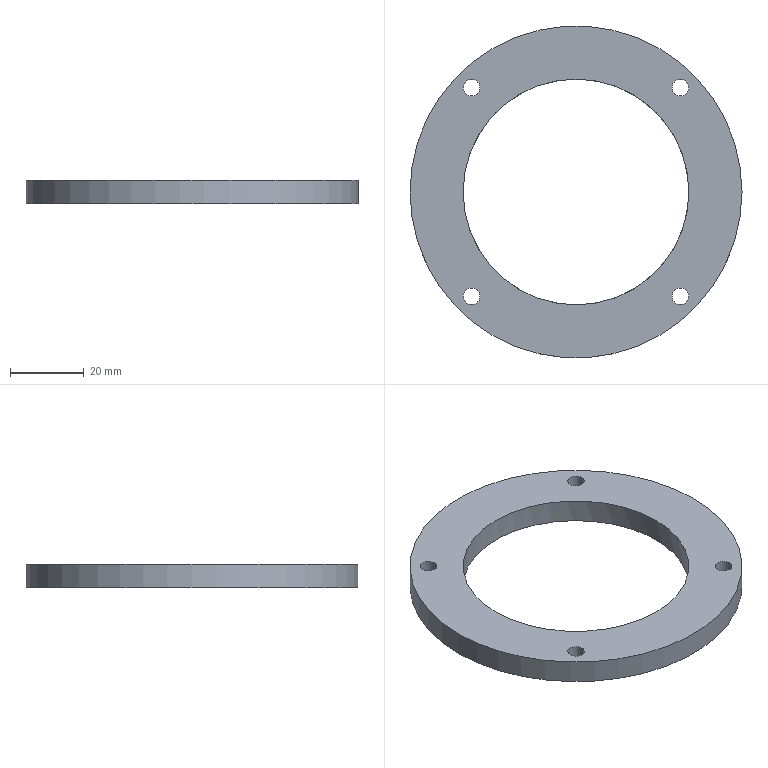Part | NX | features DATUM_CSYS 1, EXTRUDE 1, LINKED_FACE 1, SKETCH 1 | 1 solid | 8 faces | box 90 x 90 x 6.5 mm | volume 21817 mm3 | cylinder 6 | plane 2 | commonest cylinder face diameters 4.5 x4 61.2 x1 90 x1
STEP:
#1=CARTESIAN_POINT('',(-26.034,-28.284,0.));
#2=VERTEX_POINT('',#1);
#3=CARTESIAN_POINT('',(-28.284,-28.284,0.));
#4=DIRECTION('',(0.,0.,1.));
#5=DIRECTION('',(1.,0.,0.));
#6=AXIS2_PLACEMENT_3D('',#3,#4,#5);
#7=CIRCLE('',#6,2.25);
#8=EDGE_CURVE('',#2,#2,#7,.T.);
#9=ORIENTED_EDGE('',*,*,#8,.F.);
#10=EDGE_LOOP('',(#9));
#11=FACE_BOUND('',#10,.T.);
#12=CARTESIAN_POINT('',(-30.534,-28.284,6.5));
#13=VERTEX_POINT('',#12);
#14=CARTESIAN_POINT('',(-28.284,-28.284,6.5));
#15=DIRECTION('',(0.,0.,1.));
#16=DIRECTION('',(-1.,0.,0.));
#17=AXIS2_PLACEMENT_3D('',#14,#15,#16);
#18=CIRCLE('',#17,2.25);
#19=EDGE_CURVE('',#13,#13,#18,.T.);
#20=ORIENTED_EDGE('',*,*,#19,.T.);
#21=EDGE_LOOP('',(#20));
#22=FACE_BOUND('',#21,.T.);
#23=CARTESIAN_POINT('',(-28.284,-28.284,6.5));
#24=DIRECTION('',(0.,0.,-1.));
#25=DIRECTION('',(-1.,0.,0.));
#26=AXIS2_PLACEMENT_3D('',#23,#24,#25);
#27=CYLINDRICAL_SURFACE('',#26,2.25);
#28=ADVANCED_FACE('',(#11,#22),#27,.F.);
#29=CARTESIAN_POINT('',(-26.034,28.284,0.));
#30=VERTEX_POINT('',#29);
#31=CARTESIAN_POINT('',(-28.284,28.284,0.));
#32=DIRECTION('',(0.,0.,1.));
#33=DIRECTION('',(1.,0.,0.));
#34=AXIS2_PLACEMENT_3D('',#31,#32,#33);
#35=CIRCLE('',#34,2.25);
#36=EDGE_CURVE('',#30,#30,#35,.T.);
#37=ORIENTED_EDGE('',*,*,#36,.F.);
#38=EDGE_LOOP('',(#37));
#39=FACE_BOUND('',#38,.T.);
#40=CARTESIAN_POINT('',(-30.534,28.284,6.5));
#41=VERTEX_POINT('',#40);
#42=CARTESIAN_POINT('',(-28.284,28.284,6.5));
#43=DIRECTION('',(0.,0.,1.));
#44=DIRECTION('',(-1.,0.,0.));
#45=AXIS2_PLACEMENT_3D('',#42,#43,#44);
#46=CIRCLE('',#45,2.25);
#47=EDGE_CURVE('',#41,#41,#46,.T.);
#48=ORIENTED_EDGE('',*,*,#47,.T.);
#49=EDGE_LOOP('',(#48));
#50=FACE_BOUND('',#49,.T.);
#51=CARTESIAN_POINT('',(-28.284,28.284,6.5));
#52=DIRECTION('',(0.,0.,-1.));
#53=DIRECTION('',(-1.,0.,0.));
#54=AXIS2_PLACEMENT_3D('',#51,#52,#53);
#55=CYLINDRICAL_SURFACE('',#54,2.25);
#56=ADVANCED_FACE('',(#39,#50),#55,.F.);
#57=CARTESIAN_POINT('',(30.534,-28.284,0.));
#58=VERTEX_POINT('',#57);
#59=CARTESIAN_POINT('',(28.284,-28.284,0.));
#60=DIRECTION('',(0.,0.,1.));
#61=DIRECTION('',(1.,0.,0.));
#62=AXIS2_PLACEMENT_3D('',#59,#60,#61);
#63=CIRCLE('',#62,2.25);
#64=EDGE_CURVE('',#58,#58,#63,.T.);
#65=ORIENTED_EDGE('',*,*,#64,.F.);
#66=EDGE_LOOP('',(#65));
#67=FACE_BOUND('',#66,.T.);
#68=CARTESIAN_POINT('',(26.034,-28.284,6.5));
#69=VERTEX_POINT('',#68);
#70=CARTESIAN_POINT('',(28.284,-28.284,6.5));
#71=DIRECTION('',(0.,0.,1.));
#72=DIRECTION('',(-1.,0.,0.));
#73=AXIS2_PLACEMENT_3D('',#70,#71,#72);
#74=CIRCLE('',#73,2.25);
#75=EDGE_CURVE('',#69,#69,#74,.T.);
#76=ORIENTED_EDGE('',*,*,#75,.T.);
#77=EDGE_LOOP('',(#76));
#78=FACE_BOUND('',#77,.T.);
#79=CARTESIAN_POINT('',(28.284,-28.284,6.5));
#80=DIRECTION('',(0.,0.,-1.));
#81=DIRECTION('',(-1.,0.,0.));
#82=AXIS2_PLACEMENT_3D('',#79,#80,#81);
#83=CYLINDRICAL_SURFACE('',#82,2.25);
#84=ADVANCED_FACE('',(#67,#78),#83,.F.);
#85=CARTESIAN_POINT('',(30.534,28.284,0.));
#86=VERTEX_POINT('',#85);
#87=CARTESIAN_POINT('',(28.284,28.284,0.));
#88=DIRECTION('',(0.,0.,1.));
#89=DIRECTION('',(1.,0.,0.));
#90=AXIS2_PLACEMENT_3D('',#87,#88,#89);
#91=CIRCLE('',#90,2.25);
#92=EDGE_CURVE('',#86,#86,#91,.T.);
#93=ORIENTED_EDGE('',*,*,#92,.F.);
#94=EDGE_LOOP('',(#93));
#95=FACE_BOUND('',#94,.T.);
#96=CARTESIAN_POINT('',(26.034,28.284,6.5));
#97=VERTEX_POINT('',#96);
#98=CARTESIAN_POINT('',(28.284,28.284,6.5));
#99=DIRECTION('',(0.,0.,1.));
#100=DIRECTION('',(-1.,0.,0.));
#101=AXIS2_PLACEMENT_3D('',#98,#99,#100);
#102=CIRCLE('',#101,2.25);
#103=EDGE_CURVE('',#97,#97,#102,.T.);
#104=ORIENTED_EDGE('',*,*,#103,.T.);
#105=EDGE_LOOP('',(#104));
#106=FACE_BOUND('',#105,.T.);
#107=CARTESIAN_POINT('',(28.284,28.284,6.5));
#108=DIRECTION('',(0.,0.,-1.));
#109=DIRECTION('',(-1.,0.,0.));
#110=AXIS2_PLACEMENT_3D('',#107,#108,#109);
#111=CYLINDRICAL_SURFACE('',#110,2.25);
#112=ADVANCED_FACE('',(#95,#106),#111,.F.);
#113=CARTESIAN_POINT('',(-45.,0.,0.));
#114=VERTEX_POINT('',#113);
#115=CARTESIAN_POINT('',(0.,0.,0.));
#116=DIRECTION('',(0.,0.,-1.));
#117=DIRECTION('',(-1.,0.,0.));
#118=AXIS2_PLACEMENT_3D('',#115,#116,#117);
#119=CIRCLE('',#118,45.);
#120=EDGE_CURVE('',#114,#114,#119,.T.);
#121=ORIENTED_EDGE('',*,*,#120,.F.);
#122=EDGE_LOOP('',(#121));
#123=FACE_BOUND('',#122,.T.);
#124=CARTESIAN_POINT('',(45.,0.,6.5));
#125=VERTEX_POINT('',#124);
#126=CARTESIAN_POINT('',(0.,0.,6.5));
#127=DIRECTION('',(0.,0.,-1.));
#128=DIRECTION('',(1.,0.,0.));
#129=AXIS2_PLACEMENT_3D('',#126,#127,#128);
#130=CIRCLE('',#129,45.);
#131=EDGE_CURVE('',#125,#125,#130,.T.);
#132=ORIENTED_EDGE('',*,*,#131,.T.);
#133=EDGE_LOOP('',(#132));
#134=FACE_BOUND('',#133,.T.);
#135=CARTESIAN_POINT('',(0.,0.,6.5));
#136=DIRECTION('',(0.,0.,-1.));
#137=DIRECTION('',(-1.,0.,0.));
#138=AXIS2_PLACEMENT_3D('',#135,#136,#137);
#139=CYLINDRICAL_SURFACE('',#138,45.);
#140=ADVANCED_FACE('',(#123,#134),#139,.T.);
#141=CARTESIAN_POINT('',(-30.6,0.,0.));
#142=VERTEX_POINT('',#141);
#143=CARTESIAN_POINT('',(0.,0.,0.));
#144=DIRECTION('',(0.,0.,1.));
#145=DIRECTION('',(-1.,0.,0.));
#146=AXIS2_PLACEMENT_3D('',#143,#144,#145);
#147=CIRCLE('',#146,30.6);
#148=EDGE_CURVE('',#142,#142,#147,.T.);
#149=ORIENTED_EDGE('',*,*,#148,.F.);
#150=EDGE_LOOP('',(#149));
#151=FACE_BOUND('',#150,.T.);
#152=CARTESIAN_POINT('',(30.6,0.,6.5));
#153=VERTEX_POINT('',#152);
#154=CARTESIAN_POINT('',(0.,0.,6.5));
#155=DIRECTION('',(0.,0.,1.));
#156=DIRECTION('',(1.,0.,0.));
#157=AXIS2_PLACEMENT_3D('',#154,#155,#156);
#158=CIRCLE('',#157,30.6);
#159=EDGE_CURVE('',#153,#153,#158,.T.);
#160=ORIENTED_EDGE('',*,*,#159,.T.);
#161=EDGE_LOOP('',(#160));
#162=FACE_BOUND('',#161,.T.);
#163=CARTESIAN_POINT('',(0.,0.,6.5));
#164=DIRECTION('',(0.,0.,-1.));
#165=DIRECTION('',(-1.,0.,0.));
#166=AXIS2_PLACEMENT_3D('',#163,#164,#165);
#167=CYLINDRICAL_SURFACE('',#166,30.6);
#168=ADVANCED_FACE('',(#151,#162),#167,.F.);
#169=ORIENTED_EDGE('',*,*,#131,.F.);
#170=EDGE_LOOP('',(#169));
#171=FACE_BOUND('',#170,.T.);
#172=ORIENTED_EDGE('',*,*,#103,.F.);
#173=EDGE_LOOP('',(#172));
#174=FACE_BOUND('',#173,.T.);
#175=ORIENTED_EDGE('',*,*,#75,.F.);
#176=EDGE_LOOP('',(#175));
#177=FACE_BOUND('',#176,.T.);
#178=ORIENTED_EDGE('',*,*,#47,.F.);
#179=EDGE_LOOP('',(#178));
#180=FACE_BOUND('',#179,.T.);
#181=ORIENTED_EDGE('',*,*,#19,.F.);
#182=EDGE_LOOP('',(#181));
#183=FACE_BOUND('',#182,.T.);
#184=ORIENTED_EDGE('',*,*,#159,.F.);
#185=EDGE_LOOP('',(#184));
#186=FACE_BOUND('',#185,.T.);
#187=CARTESIAN_POINT('',(14.142,14.142,6.5));
#188=DIRECTION('',(0.,0.,-1.));
#189=DIRECTION('',(-1.,0.,0.));
#190=AXIS2_PLACEMENT_3D('',#187,#188,#189);
#191=PLANE('',#190);
#192=ADVANCED_FACE('',(#171,#174,#177,#180,#183,#186),#191,.F.);
#193=ORIENTED_EDGE('',*,*,#120,.T.);
#194=EDGE_LOOP('',(#193));
#195=FACE_BOUND('',#194,.T.);
#196=ORIENTED_EDGE('',*,*,#92,.T.);
#197=EDGE_LOOP('',(#196));
#198=FACE_BOUND('',#197,.T.);
#199=ORIENTED_EDGE('',*,*,#64,.T.);
#200=EDGE_LOOP('',(#199));
#201=FACE_BOUND('',#200,.T.);
#202=ORIENTED_EDGE('',*,*,#36,.T.);
#203=EDGE_LOOP('',(#202));
#204=FACE_BOUND('',#203,.T.);
#205=ORIENTED_EDGE('',*,*,#8,.T.);
#206=EDGE_LOOP('',(#205));
#207=FACE_BOUND('',#206,.T.);
#208=ORIENTED_EDGE('',*,*,#148,.T.);
#209=EDGE_LOOP('',(#208));
#210=FACE_BOUND('',#209,.T.);
#211=CARTESIAN_POINT('',(14.142,14.142,0.));
#212=DIRECTION('',(0.,0.,-1.));
#213=DIRECTION('',(-1.,0.,0.));
#214=AXIS2_PLACEMENT_3D('',#211,#212,#213);
#215=PLANE('',#214);
#216=ADVANCED_FACE('',(#195,#198,#201,#204,#207,#210),#215,.T.);
#217=CLOSED_SHELL('',(#28,#56,#84,#112,#140,#168,#192,#216));
#218=MANIFOLD_SOLID_BREP('',#217);
#219=(LENGTH_UNIT()NAMED_UNIT(*)SI_UNIT(.MILLI.,.METRE.));
#220=UNCERTAINTY_MEASURE_WITH_UNIT(LENGTH_MEASURE(0.00001),#219,'','');
#221=(NAMED_UNIT(*)PLANE_ANGLE_UNIT()SI_UNIT($,.RADIAN.));
#222=(NAMED_UNIT(*)SI_UNIT($,.STERADIAN.)SOLID_ANGLE_UNIT());
#223=(GEOMETRIC_REPRESENTATION_CONTEXT(3)GLOBAL_UNCERTAINTY_ASSIGNED_CONTEXT((#220))GLOBAL_UNIT_ASSIGNED_CONTEXT((#219,#221,#222))REPRESENTATION_CONTEXT('',''));
#224=ADVANCED_BREP_SHAPE_REPRESENTATION('',(#218),#223);